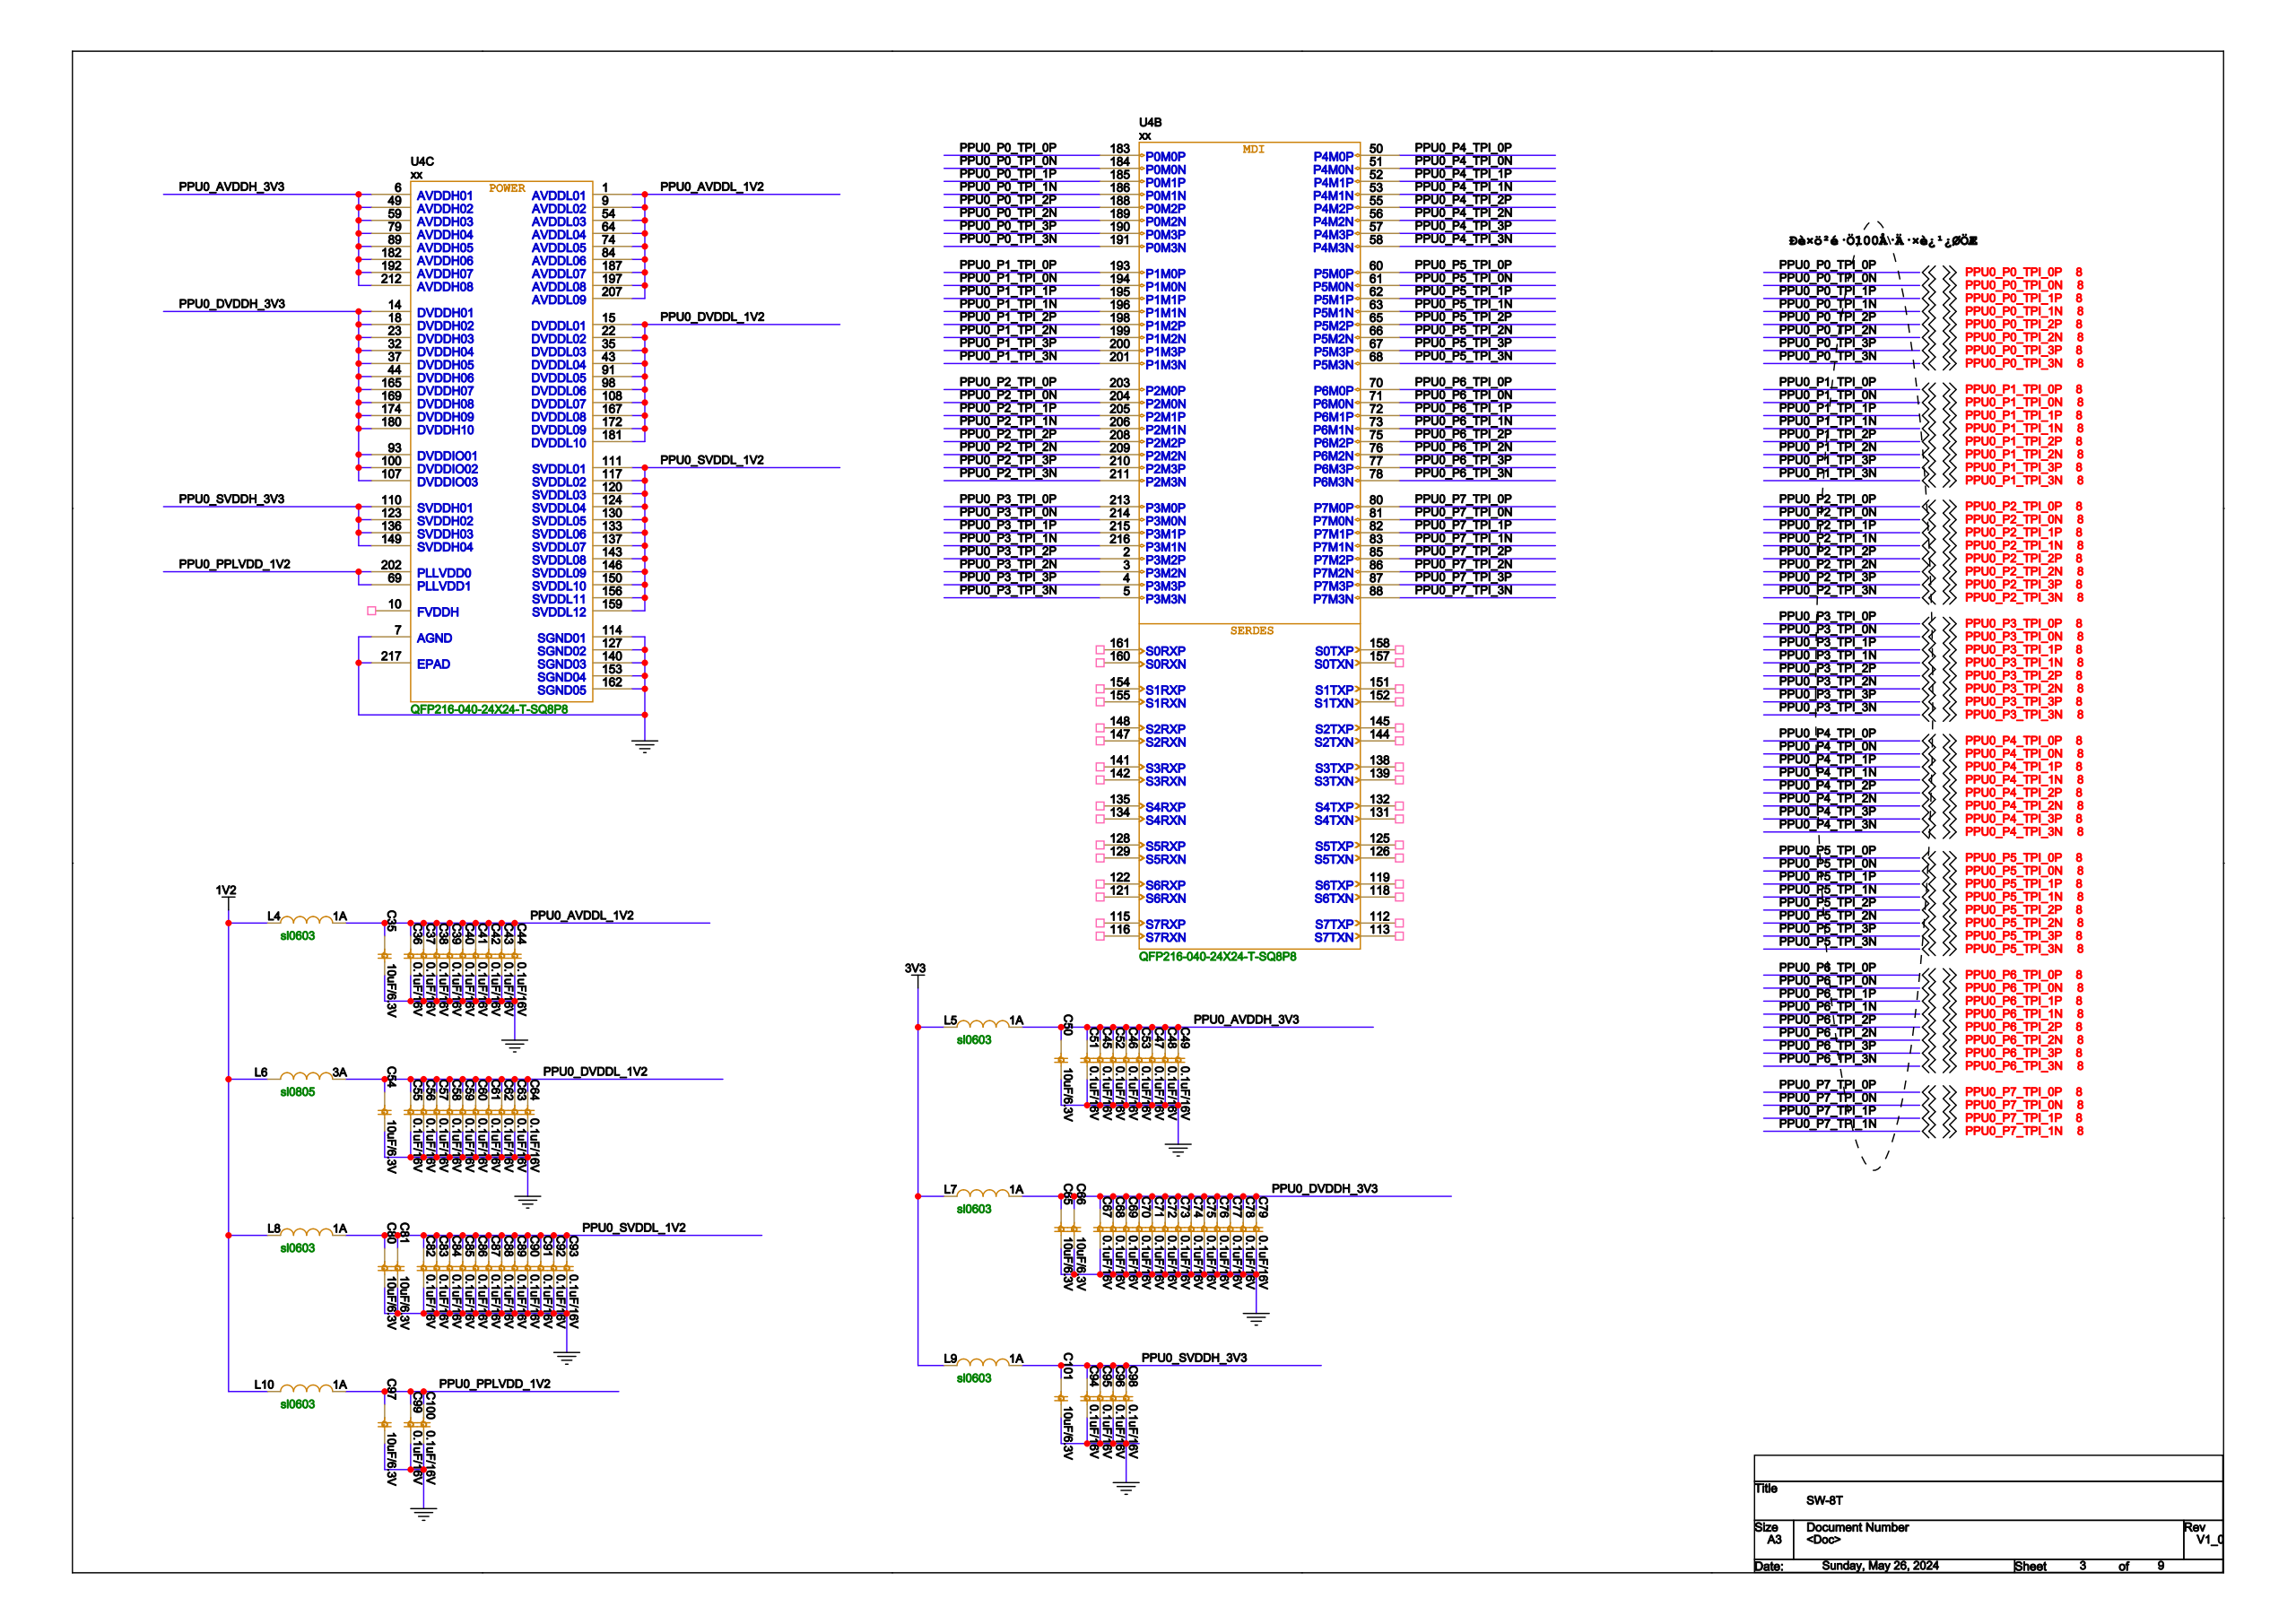Circuit board | Cadence Allegro | 399 parts | 387 nets | one sheet of the schematic
Parts on this sheet (reference | value | footprint):
C35 | 10uF/6.3V | SC0603
C36 | 0.1uF/16V | SC0402
C37 | 0.1uF/16V | SC0402
C38 | 0.1uF/16V | SC0402
C39 | 0.1uF/16V | SC0402
C40 | 0.1uF/16V | SC0402
C41 | 0.1uF/16V | SC0402
C42 | 0.1uF/16V | SC0402
C43 | 0.1uF/16V | SC0402
C44 | 0.1uF/16V | SC0402
C45 | 0.1uF/16V | SC0402
C46 | 0.1uF/16V | SC0402
C47 | 0.1uF/16V | SC0402
C48 | 0.1uF/16V | SC0402
C49 | 0.1uF/16V | SC0402
C50 | 10uF/6.3V | SC0603
C51 | 0.1uF/16V | SC0402
C52 | 0.1uF/16V | SC0402
C53 | 0.1uF/16V | SC0402
C54 | 10uF/6.3V | SC0603
C55 | 0.1uF/16V | SC0402
C56 | 0.1uF/16V | SC0402
C57 | 0.1uF/16V | SC0402
C58 | 0.1uF/16V | SC0402
C59 | 0.1uF/16V | SC0402
C60 | 0.1uF/16V | SC0402
C61 | 0.1uF/16V | SC0402
C62 | 0.1uF/16V | SC0402
C63 | 0.1uF/16V | SC0402
C64 | 0.1uF/16V | SC0402
C65 | 10uF/6.3V | SC0603
C66 | 10uF/6.3V | SC0603
C67 | 0.1uF/16V | SC0402
C68 | 0.1uF/16V | SC0402
C69 | 0.1uF/16V | SC0402
C70 | 0.1uF/16V | SC0402
C71 | 0.1uF/16V | SC0402
C72 | 0.1uF/16V | SC0402
C73 | 0.1uF/16V | SC0402
C74 | 0.1uF/16V | SC0402
C75 | 0.1uF/16V | SC0402
C76 | 0.1uF/16V | SC0402
C77 | 0.1uF/16V | SC0402
C78 | 0.1uF/16V | SC0402
C79 | 0.1uF/16V | SC0402
C80 | 10uF/6.3V | SC0603
C81 | 10uF/6.3V | SC0603
C82 | 0.1uF/16V | SC0402
C83 | 0.1uF/16V | SC0402
C84 | 0.1uF/16V | SC0402
C85 | 0.1uF/16V | SC0402
C86 | 0.1uF/16V | SC0402
C87 | 0.1uF/16V | SC0402
C88 | 0.1uF/16V | SC0402
C89 | 0.1uF/16V | SC0402
C90 | 0.1uF/16V | SC0402
C91 | 0.1uF/16V | SC0402
C92 | 0.1uF/16V | SC0402
C93 | 0.1uF/16V | SC0402
C94 | 0.1uF/16V | SC0402
C95 | 0.1uF/16V | SC0402
C96 | 0.1uF/16V | SC0402
C97 | 10uF/6.3V | SC0603
C98 | 0.1uF/16V | SC0402
C99 | 0.1uF/16V | SC0402
C100 | 0.1uF/16V | SC0402
C101 | 10uF/6.3V | SC0603
L4 | 1A | SL0603
L5 | 1A | SL0603
L6 | 3A | SL0805
L7 | 1A | SL0603
L8 | 1A | SL0603
L9 | 1A | SL0603
L10 | 1A | SL0603
U4 | xx | QFP216-040-24X24-T-SQ8P8
Nets of these parts (net: part-pin ...):
GND: C35-2 C36-2 C37-2 C38-2 C39-2 C40-2 C41-2 C42-2 C43-2 C44-2 C45-2 C46-2 C47-2 C48-2 C49-2 C50-2 C51-2 C52-2 C53-2 C54-2 C55-2 C56-2 C57-2 C58-2 C59-2 C60-2 C61-2 C62-2 C63-2 C64-2 C65-2 C66-2 C67-2 C68-2 C69-2 C70-2 C71-2 C72-2 C73-2 C74-2 C75-2 C76-2 C77-2 C78-2 C79-2 C80-2 C81-2 C82-2 C83-2 C84-2 C85-2 C86-2 C87-2 C88-2 C89-2 C90-2 C91-2 C92-2 C93-2 C94-2 C95-2 C96-2 C97-2 C98-2 C99-2 C100-2 C101-2 U4-7 U4-114 U4-127 U4-140 U4-153 U4-162 U4-217
PPU0_PPLVDD_1V2: C97-1 C99-1 C100-1 L10-2 U4-69 U4-202
3V3: L5-1 L7-1 L9-1
PPU0_AVDDL_1V2: C35-1 C36-1 C37-1 C38-1 C39-1 C40-1 C41-1 C42-1 C43-1 C44-1 L4-2 U4-1 U4-9 U4-54 U4-64 U4-74 U4-84 U4-187 U4-197 U4-207
PPU0_AVDDH_3V3: C45-1 C46-1 C47-1 C48-1 C49-1 C50-1 C51-1 C52-1 C53-1 L5-2 U4-6 U4-49 U4-59 U4-79 U4-89 U4-182 U4-192 U4-212
PPU0_DVDDL_1V2: C54-1 C55-1 C56-1 C57-1 C58-1 C59-1 C60-1 C61-1 C62-1 C63-1 C64-1 L6-2 U4-15 U4-22 U4-35 U4-43 U4-91 U4-98 U4-108 U4-167 U4-172 U4-181
PPU0_DVDDH_3V3: C65-1 C66-1 C67-1 C68-1 C69-1 C70-1 C71-1 C72-1 C73-1 C74-1 C75-1 C76-1 C77-1 C78-1 C79-1 L7-2 U4-14 U4-18 U4-23 U4-32 U4-37 U4-44 U4-93 U4-100 U4-107 U4-165 U4-169 U4-174 U4-180
PPU0_SVDDL_1V2: C80-1 C81-1 C82-1 C83-1 C84-1 C85-1 C86-1 C87-1 C88-1 C89-1 C90-1 C91-1 C92-1 C93-1 L8-2 U4-111 U4-117 U4-120 U4-124 U4-130 U4-133 U4-137 U4-143 U4-146 U4-150 U4-156 U4-159
PPU0_SVDDH_3V3: C94-1 C95-1 C96-1 C98-1 C101-1 L9-2 U4-110 U4-123 U4-136 U4-149
1V2: L4-1 L6-1 L8-1 L10-1
PPU0_P3_TPI_3N: U4-5
PPU0_P3_TPI_3P: U4-4
PPU0_P3_TPI_2N: U4-3
PPU0_P3_TPI_2P: U4-2
PPU0_P3_TPI_1N: U4-216
PPU0_P3_TPI_1P: U4-215
PPU0_P3_TPI_0N: U4-214
PPU0_P3_TPI_0P: U4-213
PPU0_P2_TPI_3N: U4-211
PPU0_P2_TPI_3P: U4-210
PPU0_P2_TPI_2N: U4-209
PPU0_P2_TPI_2P: U4-208
PPU0_P2_TPI_1N: U4-206
PPU0_P2_TPI_1P: U4-205
PPU0_P2_TPI_0N: U4-204
PPU0_P2_TPI_0P: U4-203
PPU0_P1_TPI_3N: U4-201
PPU0_P1_TPI_3P: U4-200
PPU0_P1_TPI_2N: U4-199
PPU0_P1_TPI_2P: U4-198
PPU0_P1_TPI_1N: U4-196
PPU0_P1_TPI_1P: U4-195
PPU0_P1_TPI_0N: U4-194
PPU0_P1_TPI_0P: U4-193
PPU0_P0_TPI_3N: U4-191
PPU0_P0_TPI_3P: U4-190
PPU0_P0_TPI_2N: U4-189
PPU0_P0_TPI_2P: U4-188
PPU0_P0_TPI_1N: U4-186
PPU0_P0_TPI_1P: U4-185
PPU0_P0_TPI_0N: U4-184
PPU0_P0_TPI_0P: U4-183
PPU0_P7_TPI_0P: U4-80
PPU0_P7_TPI_0N: U4-81
PPU0_P7_TPI_1P: U4-82
PPU0_P7_TPI_1N: U4-83
PPU0_P6_TPI_3N: U4-78
PPU0_P6_TPI_3P: U4-77
PPU0_P6_TPI_2N: U4-76
PPU0_P6_TPI_2P: U4-75
PPU0_P6_TPI_1N: U4-73
PPU0_P6_TPI_1P: U4-72
PPU0_P6_TPI_0N: U4-71
PPU0_P6_TPI_0P: U4-70
PPU0_P5_TPI_3N: U4-68
PPU0_P5_TPI_3P: U4-67
PPU0_P5_TPI_2N: U4-66
PPU0_P5_TPI_2P: U4-65
PPU0_P5_TPI_1N: U4-63
PPU0_P5_TPI_1P: U4-62
PPU0_P5_TPI_0N: U4-61
PPU0_P5_TPI_0P: U4-60
PPU0_P4_TPI_3N: U4-58
PPU0_P4_TPI_3P: U4-57
PPU0_P4_TPI_2N: U4-56
PPU0_P4_TPI_2P: U4-55
PPU0_P4_TPI_1N: U4-53
PPU0_P4_TPI_1P: U4-52
PPU0_P4_TPI_0N: U4-51
PPU0_P4_TPI_0P: U4-50
PPU0_P7_TPI_2N: U4-86
PPU0_P7_TPI_2P: U4-85
PPU0_P7_TPI_3N: U4-88
PPU0_P7_TPI_3P: U4-87